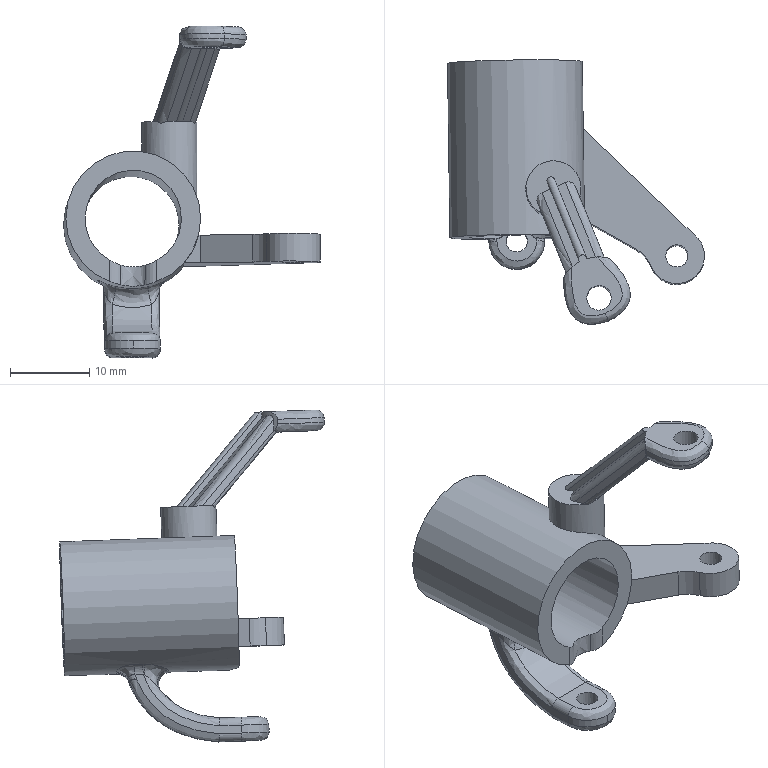Part | STEP file | Zaokr_glenie5 | 1 solid | 87 faces | box 32.405 x 33.388 x 41.862 mm | volume 3783 mm3 | spline 38 | plane 25 | cylinder 24 | commonest cylinder face diameters 2 x6 7 x3 10.348 x3 3 x2 4 x2 7.98 x2